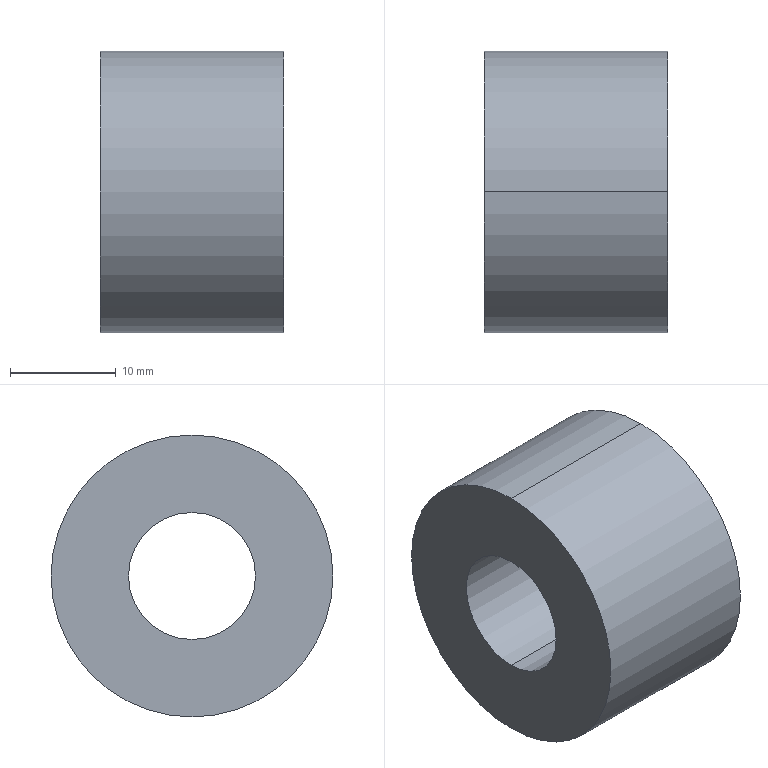Part | STEP file | 12bswbear | 1 solid | 6 faces | box 17.3 x 26.6 x 26.6 mm | volume 7657 mm3 | cylinder 4 | plane 2 | commonest cylinder face diameters 12 x2 26.6 x2
STEP:
#1=CARTESIAN_POINT('',(17.3,0.,13.3));
#2=VERTEX_POINT('',#1);
#3=CARTESIAN_POINT('',(17.3,0.,-13.3));
#4=VERTEX_POINT('',#3);
#5=CARTESIAN_POINT('',(17.3,0.,0.));
#6=DIRECTION('',(-1.,0.,0.));
#7=DIRECTION('',(0.,0.,1.));
#8=AXIS2_PLACEMENT_3D('',#5,#6,#7);
#9=CIRCLE('',#8,13.3);
#10=EDGE_CURVE('',#2,#4,#9,.T.);
#11=ORIENTED_EDGE('',*,*,#10,.T.);
#12=CARTESIAN_POINT('',(0.,0.,-13.3));
#13=VERTEX_POINT('',#12);
#14=CARTESIAN_POINT('',(10.,0.,-13.3));
#15=DIRECTION('',(-1.,0.,0.));
#16=VECTOR('',#15,1000.);
#17=LINE('',#14,#16);
#18=EDGE_CURVE('',#4,#13,#17,.T.);
#19=ORIENTED_EDGE('',*,*,#18,.T.);
#20=CARTESIAN_POINT('',(0.,0.,13.3));
#21=VERTEX_POINT('',#20);
#22=CARTESIAN_POINT('',(0.,0.,0.));
#23=DIRECTION('',(-1.,0.,0.));
#24=DIRECTION('',(0.,0.,1.));
#25=AXIS2_PLACEMENT_3D('',#22,#23,#24);
#26=CIRCLE('',#25,13.3);
#27=EDGE_CURVE('',#21,#13,#26,.T.);
#28=ORIENTED_EDGE('',*,*,#27,.F.);
#29=CARTESIAN_POINT('',(10.,0.,13.3));
#30=DIRECTION('',(-1.,0.,0.));
#31=VECTOR('',#30,1000.);
#32=LINE('',#29,#31);
#33=EDGE_CURVE('',#2,#21,#32,.T.);
#34=ORIENTED_EDGE('',*,*,#33,.F.);
#35=EDGE_LOOP('',(#11,#19,#28,#34));
#36=FACE_OUTER_BOUND('',#35,.T.);
#37=CARTESIAN_POINT('',(10.,0.,0.));
#38=DIRECTION('',(-1.,0.,0.));
#39=DIRECTION('',(0.,0.,1.));
#40=AXIS2_PLACEMENT_3D('',#37,#38,#39);
#41=CYLINDRICAL_SURFACE('',#40,13.3);
#42=ADVANCED_FACE('',(#36),#41,.T.);
#43=CARTESIAN_POINT('',(17.3,0.,-6.));
#44=VERTEX_POINT('',#43);
#45=CARTESIAN_POINT('',(17.3,0.,6.));
#46=VERTEX_POINT('',#45);
#47=CARTESIAN_POINT('',(17.3,0.,0.));
#48=DIRECTION('',(-1.,0.,0.));
#49=DIRECTION('',(0.,0.,1.));
#50=AXIS2_PLACEMENT_3D('',#47,#48,#49);
#51=CIRCLE('',#50,6.);
#52=EDGE_CURVE('',#44,#46,#51,.T.);
#53=ORIENTED_EDGE('',*,*,#52,.F.);
#54=CARTESIAN_POINT('',(0.,0.,-6.));
#55=VERTEX_POINT('',#54);
#56=CARTESIAN_POINT('',(10.,0.,-6.));
#57=DIRECTION('',(-1.,0.,0.));
#58=VECTOR('',#57,1000.);
#59=LINE('',#56,#58);
#60=EDGE_CURVE('',#44,#55,#59,.T.);
#61=ORIENTED_EDGE('',*,*,#60,.T.);
#62=CARTESIAN_POINT('',(0.,0.,6.));
#63=VERTEX_POINT('',#62);
#64=CARTESIAN_POINT('',(0.,0.,0.));
#65=DIRECTION('',(-1.,0.,0.));
#66=DIRECTION('',(0.,0.,1.));
#67=AXIS2_PLACEMENT_3D('',#64,#65,#66);
#68=CIRCLE('',#67,6.);
#69=EDGE_CURVE('',#55,#63,#68,.T.);
#70=ORIENTED_EDGE('',*,*,#69,.T.);
#71=CARTESIAN_POINT('',(10.,0.,6.));
#72=DIRECTION('',(-1.,0.,0.));
#73=VECTOR('',#72,1000.);
#74=LINE('',#71,#73);
#75=EDGE_CURVE('',#46,#63,#74,.T.);
#76=ORIENTED_EDGE('',*,*,#75,.F.);
#77=EDGE_LOOP('',(#53,#61,#70,#76));
#78=FACE_OUTER_BOUND('',#77,.T.);
#79=CARTESIAN_POINT('',(10.,0.,0.));
#80=DIRECTION('',(-1.,0.,0.));
#81=DIRECTION('',(0.,0.,1.));
#82=AXIS2_PLACEMENT_3D('',#79,#80,#81);
#83=CYLINDRICAL_SURFACE('',#82,6.);
#84=ADVANCED_FACE('',(#78),#83,.F.);
#85=CARTESIAN_POINT('',(0.,0.,0.));
#86=DIRECTION('',(-1.,0.,0.));
#87=DIRECTION('',(0.,0.,1.));
#88=AXIS2_PLACEMENT_3D('',#85,#86,#87);
#89=CIRCLE('',#88,6.);
#90=EDGE_CURVE('',#63,#55,#89,.T.);
#91=ORIENTED_EDGE('',*,*,#90,.F.);
#92=ORIENTED_EDGE('',*,*,#69,.F.);
#93=EDGE_LOOP('',(#91,#92));
#94=FACE_BOUND('',#93,.T.);
#95=ORIENTED_EDGE('',*,*,#27,.T.);
#96=CARTESIAN_POINT('',(0.,0.,0.));
#97=DIRECTION('',(-1.,0.,0.));
#98=DIRECTION('',(0.,0.,1.));
#99=AXIS2_PLACEMENT_3D('',#96,#97,#98);
#100=CIRCLE('',#99,13.3);
#101=EDGE_CURVE('',#13,#21,#100,.T.);
#102=ORIENTED_EDGE('',*,*,#101,.T.);
#103=EDGE_LOOP('',(#95,#102));
#104=FACE_OUTER_BOUND('',#103,.T.);
#105=CARTESIAN_POINT('',(0.,13.3,0.));
#106=DIRECTION('',(1.,0.,0.));
#107=DIRECTION('',(0.,0.,-1.));
#108=AXIS2_PLACEMENT_3D('',#105,#106,#107);
#109=PLANE('',#108);
#110=ADVANCED_FACE('',(#94,#104),#109,.F.);
#111=ORIENTED_EDGE('',*,*,#60,.F.);
#112=CARTESIAN_POINT('',(17.3,0.,0.));
#113=DIRECTION('',(-1.,0.,0.));
#114=DIRECTION('',(0.,0.,1.));
#115=AXIS2_PLACEMENT_3D('',#112,#113,#114);
#116=CIRCLE('',#115,6.);
#117=EDGE_CURVE('',#46,#44,#116,.T.);
#118=ORIENTED_EDGE('',*,*,#117,.F.);
#119=ORIENTED_EDGE('',*,*,#75,.T.);
#120=ORIENTED_EDGE('',*,*,#90,.T.);
#121=EDGE_LOOP('',(#111,#118,#119,#120));
#122=FACE_OUTER_BOUND('',#121,.T.);
#123=CARTESIAN_POINT('',(10.,0.,0.));
#124=DIRECTION('',(-1.,0.,0.));
#125=DIRECTION('',(0.,0.,1.));
#126=AXIS2_PLACEMENT_3D('',#123,#124,#125);
#127=CYLINDRICAL_SURFACE('',#126,6.);
#128=ADVANCED_FACE('',(#122),#127,.F.);
#129=ORIENTED_EDGE('',*,*,#10,.F.);
#130=CARTESIAN_POINT('',(17.3,0.,0.));
#131=DIRECTION('',(-1.,0.,0.));
#132=DIRECTION('',(0.,0.,1.));
#133=AXIS2_PLACEMENT_3D('',#130,#131,#132);
#134=CIRCLE('',#133,13.3);
#135=EDGE_CURVE('',#4,#2,#134,.T.);
#136=ORIENTED_EDGE('',*,*,#135,.F.);
#137=EDGE_LOOP('',(#129,#136));
#138=FACE_OUTER_BOUND('',#137,.T.);
#139=ORIENTED_EDGE('',*,*,#117,.T.);
#140=ORIENTED_EDGE('',*,*,#52,.T.);
#141=EDGE_LOOP('',(#139,#140));
#142=FACE_BOUND('',#141,.T.);
#143=CARTESIAN_POINT('',(17.3,6.,0.));
#144=DIRECTION('',(-1.,0.,0.));
#145=DIRECTION('',(0.,0.,1.));
#146=AXIS2_PLACEMENT_3D('',#143,#144,#145);
#147=PLANE('',#146);
#148=ADVANCED_FACE('',(#138,#142),#147,.F.);
#149=ORIENTED_EDGE('',*,*,#18,.F.);
#150=ORIENTED_EDGE('',*,*,#135,.T.);
#151=ORIENTED_EDGE('',*,*,#33,.T.);
#152=ORIENTED_EDGE('',*,*,#101,.F.);
#153=EDGE_LOOP('',(#149,#150,#151,#152));
#154=FACE_OUTER_BOUND('',#153,.T.);
#155=CARTESIAN_POINT('',(10.,0.,0.));
#156=DIRECTION('',(-1.,0.,0.));
#157=DIRECTION('',(0.,0.,1.));
#158=AXIS2_PLACEMENT_3D('',#155,#156,#157);
#159=CYLINDRICAL_SURFACE('',#158,13.3);
#160=ADVANCED_FACE('',(#154),#159,.T.);
#161=CLOSED_SHELL('',(#42,#84,#110,#128,#148,#160));
#162=MANIFOLD_SOLID_BREP('',#161);
#163=CARTESIAN_POINT('',(0.,0.,0.));
#164=DIRECTION('',(0.,0.,1.));
#165=DIRECTION('',(1.,0.,0.));
#166=AXIS2_PLACEMENT_3D('',#163,#164,#165);
#167=(LENGTH_UNIT()NAMED_UNIT(*)SI_UNIT(.MILLI.,.METRE.));
#168=UNCERTAINTY_MEASURE_WITH_UNIT(LENGTH_MEASURE(0.00001),#167,'','');
#169=(NAMED_UNIT(*)PLANE_ANGLE_UNIT()SI_UNIT($,.RADIAN.));
#170=(NAMED_UNIT(*)SI_UNIT($,.STERADIAN.)SOLID_ANGLE_UNIT());
#171=(GEOMETRIC_REPRESENTATION_CONTEXT(3)GLOBAL_UNCERTAINTY_ASSIGNED_CONTEXT((#168))GLOBAL_UNIT_ASSIGNED_CONTEXT((#167,#169,#170))REPRESENTATION_CONTEXT('',''));
#172=ADVANCED_BREP_SHAPE_REPRESENTATION('',(#162,#166),#171);